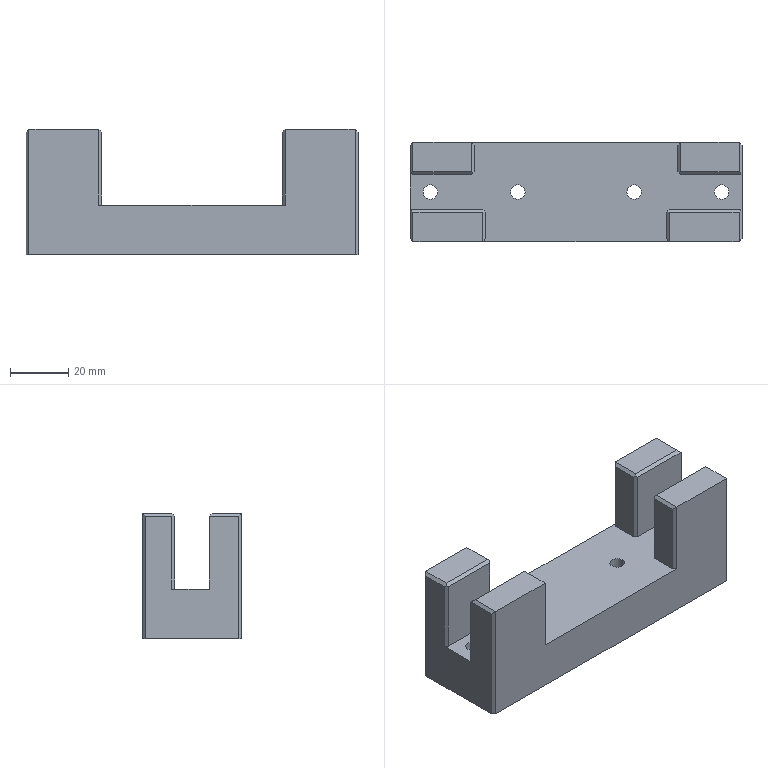CAM job | NX | 3-axis milling, drilling | part box 114 x 34 x 43 mm | stock box 114 x 34 x 43 mm
Tools:
number,name,description,diameter,corner_radius,flute_length,length,flutes
21,D17R0.8,Milling Tool-5 Parameters,17.0,0.8,50.0,75.0,2
10,D10,Milling Tool-5 Parameters,10.0,0.0,50.0,75.0,2
11,D10JING,Milling Tool-5 Parameters,10.0,0.0,50.0,75.0,2
1,ZXZ,Milling Tool-5 Parameters,6.0,0.0,50.0,75.0,2
15,5.0ZT,Drilling Tool,5.0,0.0,35.0,50.0,2
22,D6A45,Milling Tool-5 Parameters,6.0,0.0,3.0,3.0,2
Operations:
program,operation,operation_type,tool,method,geometry_group,spindle_rpm,surface_speed,feed_per_tooth,feed_cut,feed_plunge,cut_length_mm,path_length_mm,cut_time_min,machine_time_min
1虎钳,FLOOR_WALL,VolumeBased25DMillingOperation,D17R0.8,METHOD,A,2000.0,106.0,0.5,2000.0,1000.0,37166.083,38829.181,18.886,19.052
1虎钳,ZLEVEL_PROFILE_COPY,ZLevelMilling,D10,METHOD,A,3000.0,94.0,0.25,1500.0,100.0,18809.942,19533.136,12.54,12.612
1虎钳,DRILLING_COPY_1_COPY_1,Operation,ZXZ,METHOD,A,5000.0,94.0,0.025,250.0,0.0,16.0,253.412,0.064,0.0877
1虎钳,DRILLING_COPY_1_COPY_1_COPY,Operation,5.0ZT,METHOD,A,2000.0,31.0,0.0375,150.0,0.0,92.009,405.429,0.6134,0.6447
1虎钳,FLOOR_WALL_1_1_COPY,VolumeBased25DMillingOperation,D10JING,METHOD,A,7000.0,219.0,0.0714,1000.0,100.0,858.9,1366.605,0.8589,0.9097
1虎钳,ZLEVEL_PROFILE_1_COPY_1_COPY,ZLevelMilling,D6A45,METHOD,A,7500.0,141.0,0.0667,1000.0,100.0,329.242,861.253,0.3292,0.3824
1虎钳,ZLEVEL_PROFILE_1_COPY_1_COPY_COPY,ZLevelMilling,D6A45,METHOD,A,7500.0,141.0,0.0667,1000.0,100.0,315.532,739.291,0.3155,0.3579
1虎钳,ZLEVEL_PROFILE_1_COPY_1_COPY_COPY_COPY,ZLevelMilling,D6A45,METHOD,A,7500.0,141.0,0.0667,1000.0,100.0,214.456,1406.651,0.2145,0.3337
1虎钳,刀补11,ZLevelMilling,D10JING,METHOD,A,7500.0,141.0,0.0833,1250.0,100.0,461.611,1480.489,0.3693,0.4712